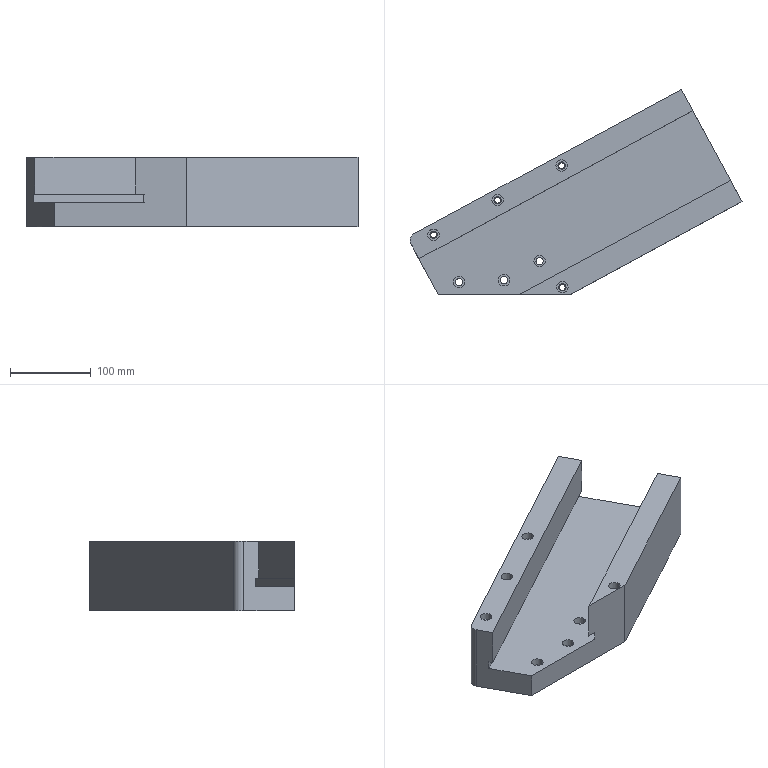Part | Creo | 1 solid | 63 faces | box 410.569 x 253.509 x 85.355 mm | volume 2672960 mm3 | cylinder 37 | plane 26 | commonest cylinder face diameters 9 x14 14.25 x14 6.985 x8 18 x1